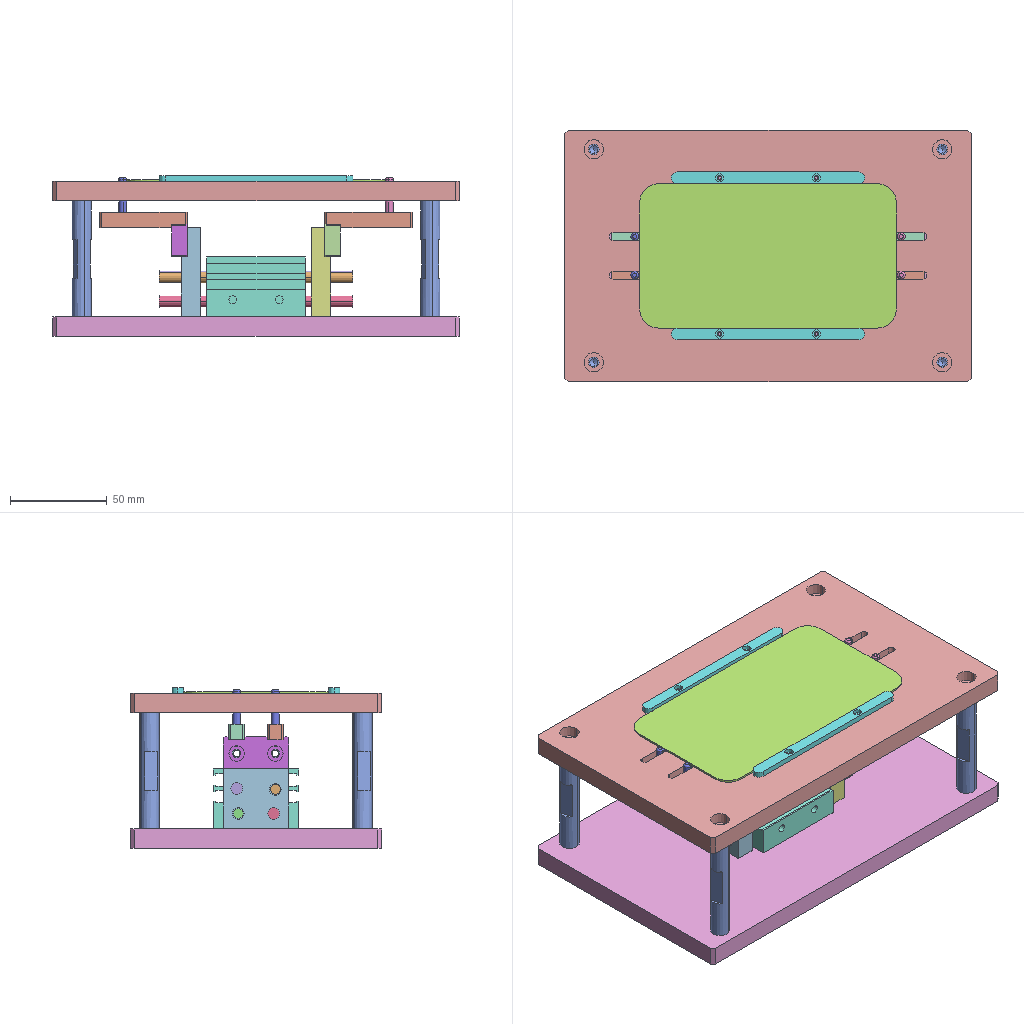Assembly | SolidWorks | 16 different items | 24 placed | box 210 x 130 x 83 mm
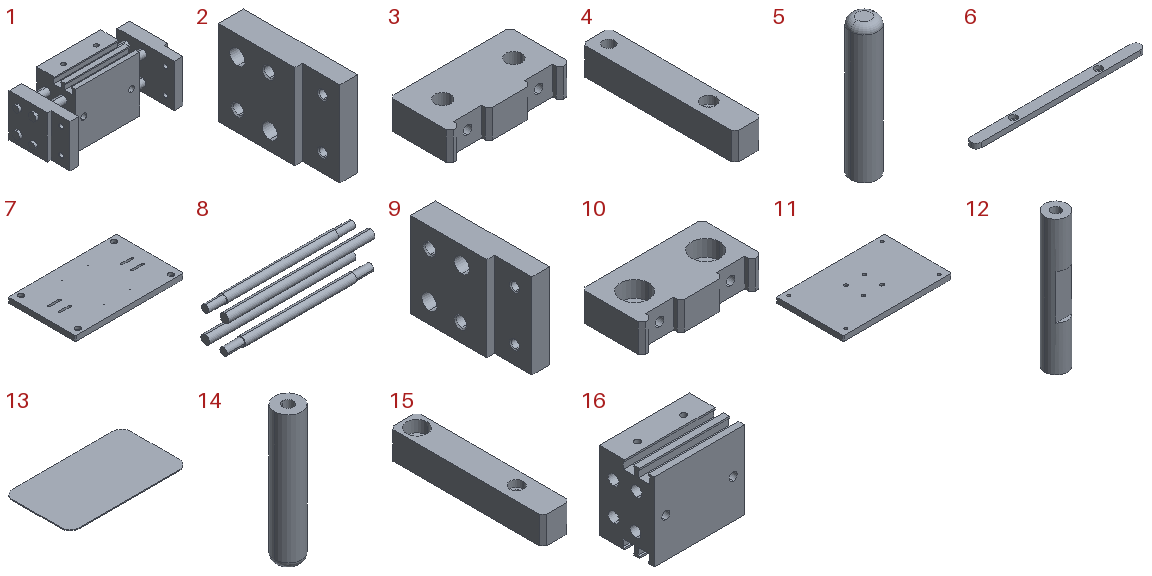Parts list (item | name | quantity | parent item | size | volume | features):
1 | (subassembly) | x1 | - | 100 x 46 x 44 mm | 92553 mm3 | -
2 | - | x1 | in 1 | 10 x 45.5 x 34 mm | 12986 mm3 | features MirrorStock 1
3 | - | x1 | - | 34 x 17 x 8 mm | 3735 mm3 | features MirrorStock 1
4 | - | x2 | - | 8 x 45 x 8 mm | 2651 mm3 | features MirrorStock 1
5 | - | x2 | - | 4 x 4 x 20 mm | 245.594 mm3 | features MirrorStock 1
6 | - | x2 | - | 100 x 6 x 3 mm | 1710 mm3 | features 3DProfileFeature 1, Extrusion 1, Fillet 1, HoleWzd 1
7 | - | x1 | - | 210 x 130 x 10 mm | 266938 mm3 | features 3DProfileFeature 2, HoleWzd 2, Chamfer 1, Cut 1, Extrusion 1
8 | - | x1 | in 1 | 100 x 19 x 26 mm | 10895 mm3 | features BaseBody 1, ICE 1
9 | - | x1 | in 1 | 10 x 45.5 x 34 mm | 12986 mm3 | features BaseBody 1
10 | - | x1 | - | 34 x 17 x 8 mm | 3735 mm3 | features 3DProfileFeature 2, HoleWzd 2, Chamfer 1, Extrusion 1, ICE 1
11 | - | x1 | - | 210 x 130 x 10 mm | 267698 mm3 | features 3DProfileFeature 2, HoleWzd 2, Chamfer 1, Extrusion 1
12 | - | x4 | - | 10 x 10 x 60 mm | 3990 mm3 | features 3DProfileFeature 1, Extrusion 1, HoleWzd 1, ICE 1, MirrorPattern 1
13 | - | x1 | - | 132.8 x 74.7 x 1 mm | 9834 mm3 | features Extrusion 1, Fillet 1
14 | - | x2 | - | 4 x 4 x 20 mm | 245.594 mm3 | features 3DProfileFeature 1, Extrusion 1, Fillet 1, HoleWzd 1
15 | - | x2 | - | 8 x 45 x 8 mm | 2651 mm3 | features 3DProfileFeature 2, HoleWzd 2, Chamfer 1, Cut 1, Extrusion 1
16 | - | x1 | in 1 | 51 x 31 x 44 mm | 55685 mm3 | features BaseBody 1
Mates (type | each side: item.copy, entity, surface, feature):
In the top assembly
Width | 7.1 face plane Boss-Extrude1 | 7.1 face plane Boss-Extrude1 | 11.1 face plane Boss-Extrude1 | 11.1 face plane Boss-Extrude1 | 2 times
Coincident | 11.1 face plane Boss-Extrude1 | 16.1 face plane Input1
Width | 11.1 face plane Boss-Extrude1 | 11.1 face plane Boss-Extrude1 | 16.1 face plane Input1 | 16.1 face plane Input1 | 2 times
DistanceDim | 11.1 face plane Boss-Extrude1 | 7.1 face plane Boss-Extrude1
Coincident | 10.1 face plane Boss-Extrude1 | 15.1 face plane Boss-Extrude1
Width | 15.1 face plane Boss-Extrude1 | 15.1 face plane Boss-Extrude1 | 7.1 face plane Cut-Extrude1 | 7.1 face plane Cut-Extrude1
Coincident | 9.1 edge | 15.1 face plane Boss-Extrude1
InPlace | 7.1 face plane Boss-Extrude1 | 6.1 plane
Coincident | 12.1 face plane Boss-Extrude1 | 11.1 face plane Boss-Extrude1
Concentric | 15.1 face cylinder Cut-Extrude1 | 14.1 face cylinder Boss-Extrude1
Coincident | 15.1 face plane Cut-Extrude1 | 14.1 face plane Boss-Extrude1
Concentric | 11.1 face cylinder Hole size (per socket head cap screw type)2 | 12.2 face cylinder Boss-Extrude1
Coincident | 9.1 face plane Input1 | 10.1 face plane Boss-Extrude1
Concentric | 9.1 face cylinder Input1 | 10.1 face cylinder Hole size (per socket head cap screw type)0
In subassembly 1
Concentric | 16.2 face cylinder Input1 | 8.1 face cylinder Input1 | 2 times
Width | 8.1 face plane Input1 | 8.1 face plane Input1 | 16.2 face plane Input1 | 16.2 face plane Input1
Concentric | 8.1 face cylinder Input1 | 9.2 face cylinder Input1 | 2 times
Concentric | 8.1 face cylinder Input1 | 2.1 face cylinder _PAX11-10-20-0-003_Mirror | 2 times
LimitDistanceDim | 9.2 face plane Input1 | 8.1 face plane Input1
LimitDistanceDim | 8.1 face plane Input1 | 2.1 face plane _PAX11-10-20-0-003_Mirror
Width | 9.2 face plane Input1 | 2.1 face plane _PAX11-10-20-0-003_Mirror | 16.2 face plane Input1 | 16.2 face plane Input1